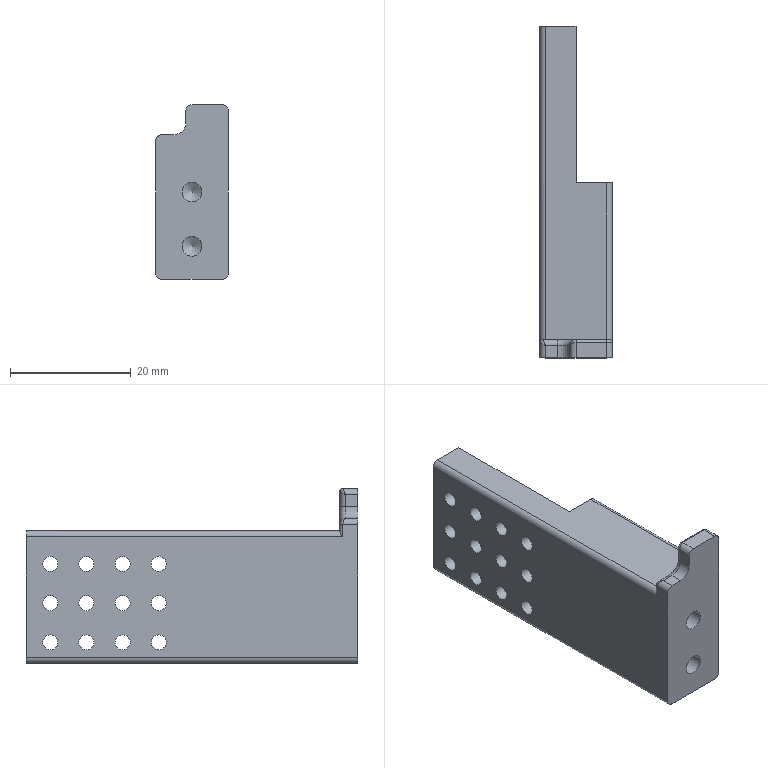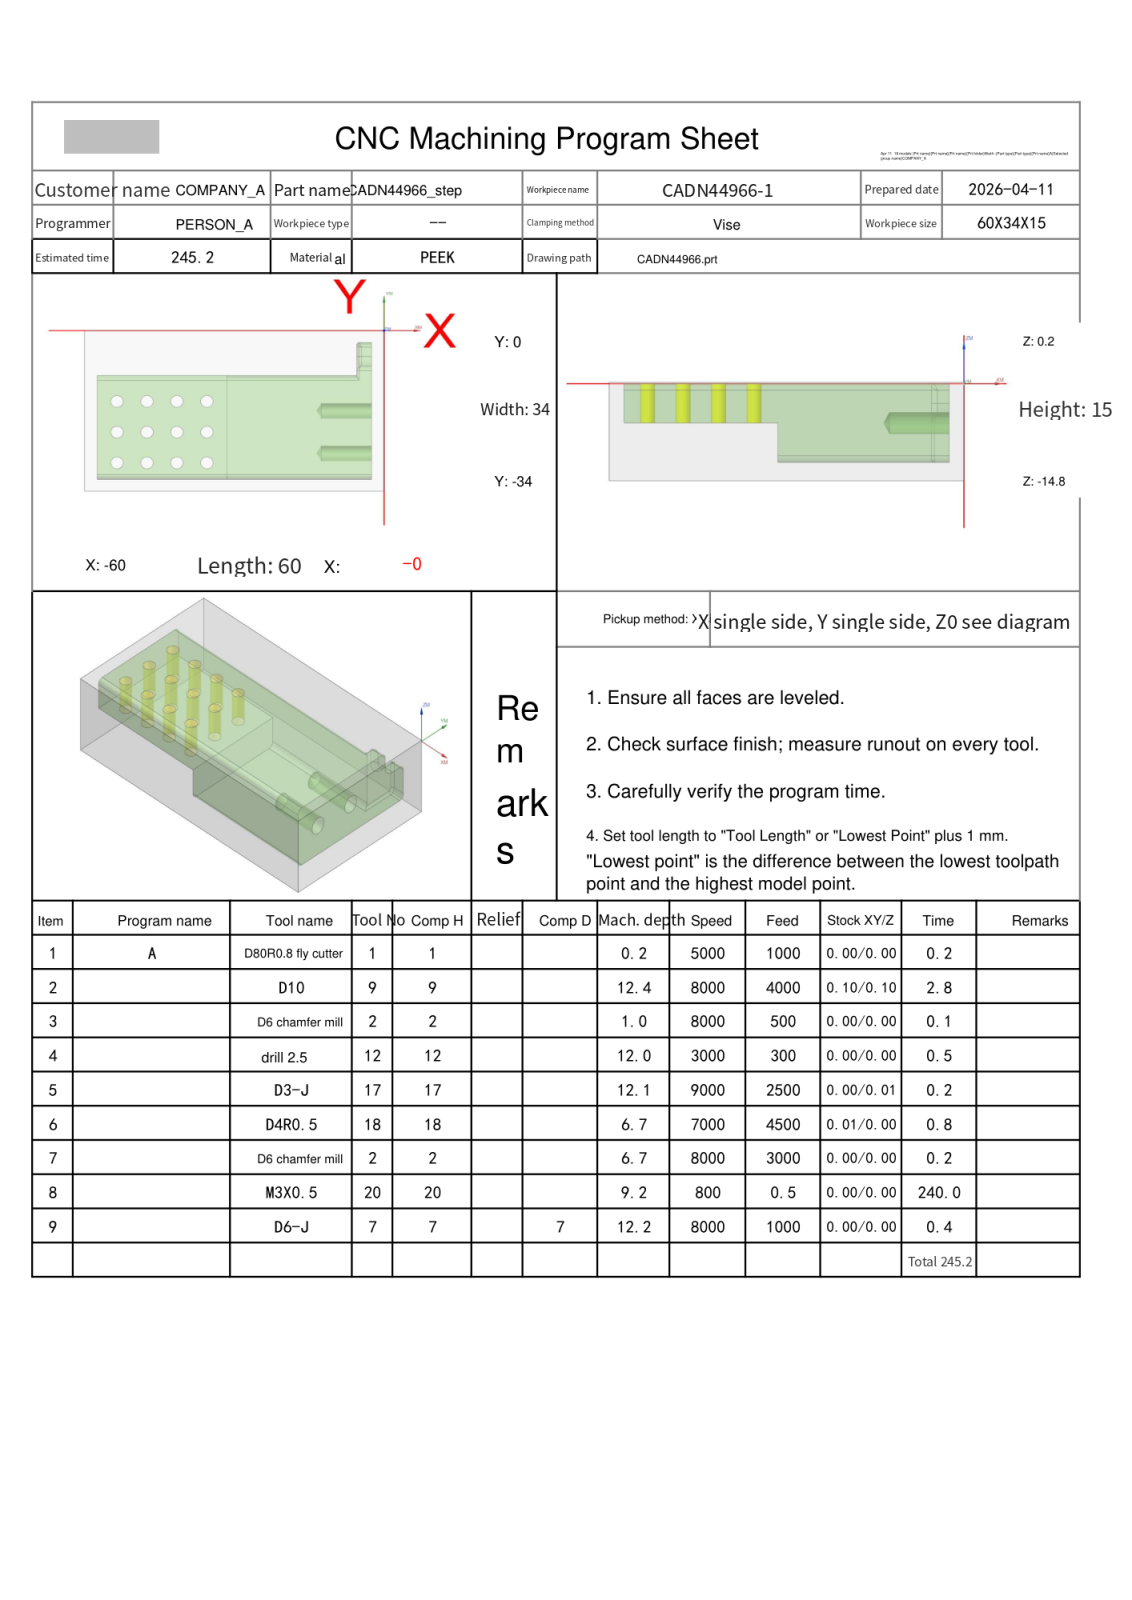NC program | NX | posted by the shop | part box 12 x 55 x 29 mm
Lines 1 to 2144 of 3281, first 1696 of 2142 lines:
%
O0001
(Machine time: 462.89 MIN)
(===Total Tool:8===)
(T1=D80R0.8 fly cutter D=80.  R=0.8  D-  H01 Z=0.    )
(T9=D10     D=10.  R=0.   D-  H09 Z=-12.2 )
(T2=D6 chamfer mill   D=6.   R=0.   D-  H02 Z=-6.5  )
(T12=drill 2.5  D=2.5  DR_a=118 D-  H12 Z=-11.75)
(T17=D3-J   D=3.   R=0.   D-  H17 Z=-11.95)
(T18=D4R0.5 D=4.   R=0.5  D-  H18 Z=-6.5  )
(T20=M3X0.5 D=2.5  DR_a=180 D-  H20 Z=-9.   )
(T7=D6-J    D=6.   R=0.   D7  H07 Z=-12.  )
G80 G90 G17 G49 G40
G91 G28 Z0
M01
N1 T01 M06
(D80R0.8 fly cutter  D=80. R=0.8 H=01 ce=0.00 di=0.00)
G00 G90 G54 X42.5 Y-17. M03 S5000
G43 H01 Z20.
M08
Z2.
G01 Z0.0 F1000.
X37.5
X-97.5
X-102.5
Z2.
G00 Z20.
G91 G28 Z0.0
M05
M09
G91 G28 Z0.0
M01
N2 T09 M06
(D10  D=10. R=0. H=09 ce=0.10 di=0.10)
G00 G90 G54 X-23.004 Y-46. M03 S8000
G43 H09 Z10.2
M08
Z.712
G01 Z-.488 F4000.
Y-44.874
G03 X-30.004 Y-37.874 I-7. J0.0
G01 X-57.509
G02 X-64. Y-31.341 I.041 J6.532
G01 Y-31.304
Y-9.696
Y-9.659
G02 X-60.5 Y-3.873 I6.533 J0.0
G01 Y0.0
G02 X-60. Y.5 I.5 J0.0
G01 X0.0
G02 X.5 Y0.0 I0.0 J-.5
G01 Y-1.869
G02 X4. Y-7.639 I-3.023 J-5.78
G01 Y-31.36
Y-31.367
G02 X-2.5 Y-37.874 I-6.506 J0.0
G01 X-35.004
G02 X-35.462 Y-37.511 I0.0 J.47
G01 X-35.524 Y-37.245
G03 X-36.497 Y-36.474 I-.974 J-.228
G01 X-57.5
G02 X-62.6 Y-31.341 I.033 J5.132
G01 Y-31.309
Y-9.692
Y-9.659
G02 X-57.5 Y-4.526 I5.133 J0.0
G01 X-9.108
G02 X-4.732 Y-2.526 I4.449 J-3.947
G01 X-2.5
G02 X2.6 Y-7.639 I-.023 J-5.123
G01 Y-31.361
Y-31.367
G02 X-2.5 Y-36.474 I-5.106 J0.0
G01 X-35.004
X-35.504
G03 X-42.504 Y-43.474 I0.0 J-7.
G01 Y-46.
Z.712
G00 Z3.
G01 X-23. F6000.
G00 Z.224
G01 Z-.976 F4000.
Y-45.
G03 X-30. Y-38. I-7. J0.0
G01 X-57.5
G02 X-64. Y-31.5 I0.0 J6.5
G01 Y-9.5
G02 X-60.5 Y-3.734 I6.5 J0.0
G01 Y0.0
G02 X-60. Y.5 I.5 J0.0
G01 X0.0
G02 X.5 Y0.0 I0.0 J-.5
G01 Y-1.735
G02 X4. Y-7.501 I-3.002 J-5.768
G01 Y-31.499
G02 X-2.5 Y-38. I-6.5 J0.0
G01 X-35.
G02 X-35.457 Y-37.637 I0.0 J.47
G01 X-35.519 Y-37.371
G03 X-36.493 Y-36.6 I-.974 J-.228
G01 X-57.5
G02 X-62.6 Y-31.5 I0.0 J5.1
G01 Y-9.5
G02 X-57.5 Y-4.4 I5.1 J0.0
G01 X-9.017
G02 X-4.793 Y-2.407 I4.517 J-4.1
G01 X-4.511 Y-2.4
X-2.504
X-2.502
G02 X2.6 Y-7.501 I0.0 J-5.102
G01 Y-31.499
G02 X-2.5 Y-36.6 I-5.1 J0.0
G01 X-35.
X-35.5
G03 X-42.5 Y-43.6 I0.0 J-7.
G01 Y-46.
Z.224
G00 Z2.512
G01 X-23. F6000.
G00 Z-.264
G01 Z-1.464 F4000.
Y-45.
G03 X-30. Y-38. I-7. J0.0
G01 X-57.5
G02 X-64. Y-31.5 I0.0 J6.5
G01 Y-9.5
G02 X-60.5 Y-3.734 I6.5 J0.0
G01 Y0.0
G02 X-60. Y.5 I.5 J0.0
G01 X0.0
G02 X.5 Y0.0 I0.0 J-.5
G01 Y-1.734
G02 X3.831 Y-6.028 I-3. J-5.766
X4. Y-7.5 I-6.331 J-1.472
G01 Y-31.5
G02 X-2.5 Y-38. I-6.5 J0.0
G01 X-35.
G02 X-35.457 Y-37.637 I0.0 J.47
G01 X-35.519 Y-37.372
G03 X-36.493 Y-36.6 I-.974 J-.228
G01 X-57.5
G02 X-62.6 Y-31.5 I0.0 J5.1
G01 Y-9.5
G02 X-57.5 Y-4.4 I5.1 J0.0
G01 X-9.017
G02 X-4.5 Y-2.4 I4.517 J-4.1
G01 X-2.5
G02 X-1.191 Y-2.571 I0.0 J-5.1
X2.467 Y-6.345 I-1.309 J-4.929
X2.6 Y-7.5 I-4.967 J-1.155
G01 Y-31.5
G02 X-2.5 Y-36.6 I-5.1 J0.0
G01 X-35.
X-35.5
G03 X-42.5 Y-43.6 I0.0 J-7.
G01 Y-46.
Z-.264
G00 Z2.024
G01 X-23. F6000.
G00 Z-.752
G01 Z-1.952 F4000.
Y-45.
G03 X-30. Y-38. I-7. J0.0
G01 X-57.5
G02 X-64. Y-31.5 I0.0 J6.5
G01 Y-9.5
G02 X-60.5 Y-3.734 I6.5 J0.0
G01 Y0.0
G02 X-60. Y.5 I.5 J0.0
G01 X0.0
G02 X.5 Y0.0 I0.0 J-.5
G01 Y-1.734
G02 X3.831 Y-6.028 I-3. J-5.766
X4. Y-7.5 I-6.331 J-1.472
G01 Y-31.5
G02 X-2.5 Y-38. I-6.5 J0.0
G01 X-35.
G02 X-35.457 Y-37.637 I0.0 J.47
G01 X-35.519 Y-37.372
G03 X-36.493 Y-36.6 I-.974 J-.228
G01 X-57.5
G02 X-62.6 Y-31.5 I0.0 J5.1
G01 Y-9.5
G02 X-57.5 Y-4.4 I5.1 J0.0
G01 X-9.017
G02 X-4.5 Y-2.4 I4.517 J-4.1
G01 X-2.5
G02 X-1.191 Y-2.571 I0.0 J-5.1
X2.467 Y-6.345 I-1.309 J-4.929
X2.6 Y-7.5 I-4.967 J-1.155
G01 Y-31.5
G02 X-2.5 Y-36.6 I-5.1 J0.0
G01 X-35.
X-35.5
G03 X-42.5 Y-43.6 I0.0 J-7.
G01 Y-46.
Z-.752
G00 Z1.536
G01 X-23. F6000.
G00 Z-1.24
G01 Z-2.44 F4000.
Y-45.
G03 X-30. Y-38. I-7. J0.0
G01 X-57.5
G02 X-64. Y-31.5 I0.0 J6.5
G01 Y-9.5
G02 X-60.5 Y-3.734 I6.5 J0.0
G01 Y0.0
G02 X-60. Y.5 I.5 J0.0
G01 X0.0
G02 X.5 Y0.0 I0.0 J-.5
G01 Y-1.734
G02 X3.831 Y-6.028 I-3. J-5.766
X4. Y-7.5 I-6.331 J-1.472
G01 Y-31.5
G02 X-2.5 Y-38. I-6.5 J0.0
G01 X-35.
G02 X-35.457 Y-37.637 I0.0 J.47
G01 X-35.519 Y-37.372
G03 X-36.493 Y-36.6 I-.974 J-.228
G01 X-57.5
G02 X-62.6 Y-31.5 I0.0 J5.1
G01 Y-9.5
G02 X-57.5 Y-4.4 I5.1 J0.0
G01 X-9.017
G02 X-4.5 Y-2.4 I4.517 J-4.1
G01 X-2.5
G02 X-1.191 Y-2.571 I0.0 J-5.1
X2.467 Y-6.345 I-1.309 J-4.929
X2.6 Y-7.5 I-4.967 J-1.155
G01 Y-31.5
G02 X-2.5 Y-36.6 I-5.1 J0.0
G01 X-35.
X-35.5
G03 X-42.5 Y-43.6 I0.0 J-7.
G01 Y-46.
Z-1.24
G00 Z1.048
G01 X-23. F6000.
G00 Z-1.728
G01 Z-2.928 F4000.
Y-45.
G03 X-30. Y-38. I-7. J0.0
G01 X-57.5
G02 X-64. Y-31.5 I0.0 J6.5
G01 Y-9.5
G02 X-60.5 Y-3.734 I6.5 J0.0
G01 Y0.0
G02 X-60. Y.5 I.5 J0.0
G01 X0.0
G02 X.5 Y0.0 I0.0 J-.5
G01 Y-1.734
G02 X3.831 Y-6.028 I-3. J-5.766
X4. Y-7.5 I-6.331 J-1.472
G01 Y-31.5
G02 X-2.5 Y-38. I-6.5 J0.0
G01 X-35.
G02 X-35.457 Y-37.637 I0.0 J.47
G01 X-35.519 Y-37.372
G03 X-36.493 Y-36.6 I-.974 J-.228
G01 X-57.5
G02 X-62.6 Y-31.5 I0.0 J5.1
G01 Y-9.5
G02 X-57.5 Y-4.4 I5.1 J0.0
G01 X-9.017
G02 X-4.5 Y-2.4 I4.517 J-4.1
G01 X-2.5
G02 X-1.191 Y-2.571 I0.0 J-5.1
X2.467 Y-6.345 I-1.309 J-4.929
X2.6 Y-7.5 I-4.967 J-1.155
G01 Y-31.5
G02 X-2.5 Y-36.6 I-5.1 J0.0
G01 X-35.
X-35.5
G03 X-42.5 Y-43.6 I0.0 J-7.
G01 Y-46.
Z-1.728
G00 Z.56
G01 X-23. F6000.
G00 Z-2.216
G01 Z-3.416 F4000.
Y-45.
G03 X-30. Y-38. I-7. J0.0
G01 X-57.5
G02 X-64. Y-31.5 I0.0 J6.5
G01 Y-9.5
G02 X-60.5 Y-3.734 I6.5 J0.0
G01 Y0.0
G02 X-60. Y.5 I.5 J0.0
G01 X0.0
G02 X.5 Y0.0 I0.0 J-.5
G01 Y-1.663
G02 X3.108 Y-4.152 I-2.927 J-5.678
X4. Y-7.413 I-5.511 J-3.261
G01 Y-7.459
Y-31.5
G02 X-2.5 Y-38. I-6.5 J0.0
G01 X-35.
G02 X-35.457 Y-37.637 I0.0 J.47
G01 X-35.519 Y-37.372
G03 X-36.493 Y-36.6 I-.974 J-.228
G01 X-57.5
G02 X-62.6 Y-31.5 I0.0 J5.1
G01 Y-9.5
G02 X-57.5 Y-4.4 I5.1 J0.0
G01 X-9.053
G02 X-4.523 Y-2.354 I4.53 J-3.991
G01 X-4.5
X-2.5
X-2.427 Y-2.353
G02 X1.899 Y-4.858 I0.0 J-4.988
X2.6 Y-7.413 I-4.302 J-2.555
G01 Y-7.454
Y-31.5
G02 X-2.5 Y-36.6 I-5.1 J0.0
G01 X-35.
X-35.5
G03 X-42.5 Y-43.6 I0.0 J-7.
G01 Y-46.
Z-2.216
G00 Z.072
G01 X-23. F6000.
G00 Z-2.704
G01 Z-3.904 F4000.
Y-45.
G03 X-30. Y-38. I-7. J0.0
G01 X-57.5
G02 X-64. Y-31.5 I0.0 J6.5
G01 Y-9.5
G02 X-60.5 Y-3.734 I6.5 J0.0
G01 Y0.0
G02 X-60. Y.5 I.5 J0.0
G01 X0.0
G02 X.5 Y0.0 I0.0 J-.5
G01 Y-1.486
G02 X4.003 Y-7.256 I-3. J-5.77
G01 X4. Y-7.454
Y-31.5
G02 X-2.5 Y-38. I-6.5 J0.0
G01 X-35.
G02 X-35.457 Y-37.637 I0.0 J.47
G01 X-35.519 Y-37.372
G03 X-36.493 Y-36.6 I-.974 J-.228
G01 X-57.5
G02 X-62.6 Y-31.5 I0.0 J5.1
G01 Y-9.5
G02 X-57.5 Y-4.4 I5.1 J0.0
G01 X-9.194
G02 X-4.516 Y-2.171 I4.678 J-3.795
G01 X-4.5
X-2.5
X-2.46 Y-2.148
X-1.864 Y-2.192
G02 X-.146 Y-2.728 I-.636 J-5.06
X2.604 Y-7.257 I-2.354 J-4.529
G01 X2.6 Y-7.454
Y-31.5
G02 X-2.5 Y-36.6 I-5.1 J0.0
G01 X-35.
X-35.5
G03 X-42.5 Y-43.6 I0.0 J-7.
G01 Y-46.
Z-2.704
G00 Z-.416
G01 X-23. F6000.
G00 Z-3.192
G01 Z-4.392 F4000.
Y-45.
G03 X-30. Y-38. I-7. J0.0
G01 X-57.5
G02 X-64. Y-31.5 I0.0 J6.5
G01 Y-9.5
G02 X-60.5 Y-3.734 I6.5 J0.0
G01 Y0.0
G02 X-60. Y.5 I.5 J0.0
G01 X0.0
G02 X.5 Y0.0 I0.0 J-.5
G01 Y-1.116
G02 X4. Y-6.867 I-2.974 J-5.751
G01 Y-6.941
Y-31.5
G02 X-2.5 Y-38. I-6.5 J0.0
G01 X-35.
G02 X-35.457 Y-37.637 I0.0 J.47
G01 X-35.519 Y-37.372
G03 X-36.493 Y-36.6 I-.974 J-.228
G01 X-57.5
G02 X-62.6 Y-31.5 I0.0 J5.1
G01 Y-9.5
G02 X-57.5 Y-4.4 I5.1 J0.0
G01 X-9.402
G02 X-4.543 Y-1.793 I4.859 J-3.225
G01 X-4.5
X-2.5
X-2.474
G02 X2.6 Y-6.867 I0.0 J-5.074
G01 Y-6.932
Y-31.5
G02 X-2.5 Y-36.6 I-5.1 J0.0
G01 X-35.
X-35.5
G03 X-42.5 Y-43.6 I0.0 J-7.
G01 Y-46.
Z-3.192
G00 Z-.904
G01 X-23. F6000.
G00 Z-3.68
G01 Z-4.88 F4000.
Y-45.
G03 X-30. Y-38. I-7. J0.0
G01 X-57.5
G02 X-64. Y-31.5 I0.0 J6.5
G01 Y-9.5
G02 X-60.5 Y-3.734 I6.5 J0.0
G01 Y0.0
G02 X-60. Y.5 I.5 J0.0
G01 X-5.654
G02 X-4.5 Y.625 I1.361 J-7.172
G01 X-2.462
G02 X-1.349 Y.5 I-.18 J-6.642
G01 X0.0
G02 X.5 Y0.0 I0.0 J-.5
G01 Y-.163
G02 X4.002 Y-6.017 I-3.142 J-5.854
G01 X4. Y-6.177
Y-31.5
G02 X-2.5 Y-38. I-6.5 J0.0
G01 X-35.
G02 X-35.457 Y-37.637 I0.0 J.47
G01 X-35.519 Y-37.372
G03 X-36.493 Y-36.6 I-.974 J-.228
G01 X-57.5
G02 X-62.6 Y-31.5 I0.0 J5.1
G01 Y-9.5
G02 X-57.5 Y-4.4 I5.1 J0.0
G01 X-9.734
G02 X-4.5 Y-.775 I5.446 J-2.272
G01 X-2.5
G02 X2.602 Y-6.017 I-.142 J-5.242
G01 X2.6 Y-6.159
Y-31.5
G02 X-2.5 Y-36.6 I-5.1 J0.0
G01 X-35.
X-35.5
G03 X-42.5 Y-43.6 I0.0 J-7.
G01 Y-46.
Z-3.68
G00 Z-1.392
G01 X-23. F6000.
G00 Z-4.168
G01 Z-5.368 F4000.
Y-45.
G03 X-30. Y-38. I-7. J0.0
G01 X-57.5
G02 X-64. Y-31.5 I0.0 J6.5
G01 Y-9.5
G02 X-60.5 Y-3.734 I6.5 J0.0
G01 Y0.0
G02 X-60. Y.5 I.5 J0.0
G01 X-10.791
G02 X-4.909 Y3.8 I5.882 J-3.591
G01 X-2.497
G02 X4. Y-2.712 I-.016 J-6.513
G01 Y-2.727
Y-5.857
X4.002 Y-6.017
X4. Y-6.177
Y-31.5
G02 X-2.5 Y-38. I-6.5 J0.0
G01 X-35.
G02 X-35.457 Y-37.637 I0.0 J.47
G01 X-35.519 Y-37.372
G03 X-36.493 Y-36.6 I-.974 J-.228
G01 X-57.5
G02 X-62.6 Y-31.5 I0.0 J5.1
G01 Y-9.5
G02 X-57.5 Y-4.4 I5.1 J0.0
G01 X-10.4
Y-3.091
G02 X-4.909 Y2.4 I5.492 J0.0
G01 X-2.5
G02 X2.6 Y-2.712 I-.013 J-5.113
G01 Y-2.725
Y-5.875
X2.602 Y-6.017
X2.6 Y-6.159
Y-31.5
G02 X-2.5 Y-36.6 I-5.1 J0.0
G01 X-35.
X-35.5
G03 X-42.5 Y-43.6 I0.0 J-7.
G01 Y-46.
Z-4.168
G00 Z-1.88
G01 X-23. F6000.
G00 Z-4.656
G01 Z-5.856 F4000.
Y-45.
G03 X-30. Y-38. I-7. J0.0
G01 X-57.5
G02 X-64. Y-31.5 I0.0 J6.5
G01 Y-9.5
G02 X-60.5 Y-3.734 I6.5 J0.0
G01 Y0.0
G02 X-60. Y.5 I.5 J0.0
G01 X-11.029
G02 X-4.996 Y3.991 I6.083 J-3.554
G01 X-2.5
G02 X4. Y-2.51 I0.0 J-6.5
G01 Y-5.857
X4.002 Y-6.017
X4. Y-6.177
Y-31.5
G02 X-2.5 Y-38. I-6.5 J0.0
G01 X-35.
G02 X-35.457 Y-37.637 I0.0 J.47
G01 X-35.519 Y-37.372
G03 X-36.493 Y-36.6 I-.974 J-.228
G01 X-57.5
G02 X-62.6 Y-31.5 I0.0 J5.1
G01 Y-9.5
G02 X-57.5 Y-4.4 I5.1 J0.0
G01 X-10.591
Y-3.004
G02 X-4.996 Y2.591 I5.645 J-.05
G01 X-2.5
G02 X2.6 Y-2.51 I0.0 J-5.1
G01 Y-5.875
X2.602 Y-6.017
X2.6 Y-6.159
Y-31.5
G02 X-2.5 Y-36.6 I-5.1 J0.0
G01 X-35.
X-35.5
G03 X-42.5 Y-43.6 I0.0 J-7.
G01 Y-46.
Z-4.656
G00 Z-2.368
G01 X-23. F6000.
G00 Z-5.144
G01 Z-6.344 F4000.
Y-45.
G03 X-30. Y-38. I-7. J0.0
G01 X-57.5
G02 X-64. Y-31.5 I0.0 J6.5
G01 Y-9.5
G02 X-60.5 Y-3.734 I6.5 J0.0
G01 Y0.0
G02 X-60. Y.5 I.5 J0.0
G01 X-11.062
G02 X-5. Y4. I6.062 J-3.5
G01 X-2.5
G02 X4. Y-2.5 I0.0 J-6.5
G01 Y-31.5
G02 X-2.5 Y-38. I-6.5 J0.0
G01 X-35.
G02 X-35.457 Y-37.637 I0.0 J.47
G01 X-35.519 Y-37.372
G03 X-36.493 Y-36.6 I-.974 J-.228
G01 X-57.5
G02 X-62.6 Y-31.5 I0.0 J5.1
G01 Y-9.5
G02 X-57.5 Y-4.4 I5.1 J0.0
G01 X-10.6
Y-3.
G02 X-5. Y2.6 I5.6 J0.0
G01 X-2.5
G02 X2.6 Y-2.5 I0.0 J-5.1
G01 Y-31.5
G02 X-2.5 Y-36.6 I-5.1 J0.0
G01 X-35.
X-35.5
G03 X-42.5 Y-43.6 I0.0 J-7.
G01 Y-46.
Z-5.144
G00 Z-2.856
G01 X-23. F6000.
G00 Z-5.632
G01 Z-6.832 F4000.
Y-45.
G03 X-30. Y-38. I-7. J0.0
G01 X-57.5
G02 X-64. Y-31.5 I0.0 J6.5
G01 Y-9.5
G02 X-60.5 Y-3.734 I6.5 J0.0
G01 Y0.0
G02 X-60. Y.5 I.5 J0.0
G01 X-11.062
G02 X-5. Y4. I6.062 J-3.5
G01 X-2.5
G02 X4. Y-2.5 I0.0 J-6.5
G01 Y-31.5
G02 X-2.5 Y-38. I-6.5 J0.0
G01 X-35.
G02 X-35.457 Y-37.637 I0.0 J.47
G01 X-35.519 Y-37.372
G03 X-36.493 Y-36.6 I-.974 J-.228
G01 X-57.5
G02 X-62.6 Y-31.5 I0.0 J5.1
G01 Y-9.5
G02 X-57.5 Y-4.4 I5.1 J0.0
G01 X-10.6
Y-3.
G02 X-5. Y2.6 I5.6 J0.0
G01 X-2.5
G02 X2.6 Y-2.5 I0.0 J-5.1
G01 Y-31.5
G02 X-2.5 Y-36.6 I-5.1 J0.0
G01 X-35.
X-35.5
G03 X-42.5 Y-43.6 I0.0 J-7.
G01 Y-46.
Z-5.632
G00 Z-3.344
G01 X-23. F6000.
G00 Z-6.12
G01 Z-7.32 F4000.
Y-45.
G03 X-30. Y-38. I-7. J0.0
G01 X-57.5
G02 X-64. Y-31.5 I0.0 J6.5
G01 Y-9.5
G02 X-60.5 Y-3.734 I6.5 J0.0
G01 Y0.0
G02 X-60. Y.5 I.5 J0.0
G01 X-11.062
G02 X-5. Y4. I6.062 J-3.5
G01 X-2.5
G02 X4. Y-2.5 I0.0 J-6.5
G01 Y-31.5
G02 X-2.5 Y-38. I-6.5 J0.0
G01 X-35.
G02 X-35.457 Y-37.637 I0.0 J.47
G01 X-35.519 Y-37.372
G03 X-36.493 Y-36.6 I-.974 J-.228
G01 X-57.5
G02 X-62.6 Y-31.5 I0.0 J5.1
G01 Y-9.5
G02 X-57.5 Y-4.4 I5.1 J0.0
G01 X-10.6
Y-3.
G02 X-5. Y2.6 I5.6 J0.0
G01 X-2.5
G02 X2.6 Y-2.5 I0.0 J-5.1
G01 Y-31.5
G02 X-2.5 Y-36.6 I-5.1 J0.0
G01 X-35.
X-35.5
G03 X-42.5 Y-43.6 I0.0 J-7.
G01 Y-46.
Z-6.12
G00 Z-3.832
G01 X-23. F6000.
G00 Z-6.608
G01 Z-7.808 F4000.
Y-45.
G03 X-30. Y-38. I-7. J0.0
G01 X-57.5
G02 X-64. Y-31.5 I0.0 J6.5
G01 Y-9.5
G02 X-60.5 Y-3.734 I6.5 J0.0
G01 Y0.0
G02 X-60. Y.5 I.5 J0.0
G01 X-11.062
G02 X-5. Y4. I6.062 J-3.5
G01 X-2.5
G02 X4. Y-2.5 I0.0 J-6.5
G01 Y-31.5
G02 X-2.5 Y-38. I-6.5 J0.0
G01 X-35.
G02 X-35.457 Y-37.637 I0.0 J.47
G01 X-35.519 Y-37.372
G03 X-36.493 Y-36.6 I-.974 J-.228
G01 X-57.5
G02 X-62.6 Y-31.5 I0.0 J5.1
G01 Y-9.5
G02 X-57.5 Y-4.4 I5.1 J0.0
G01 X-10.6
Y-3.
G02 X-5. Y2.6 I5.6 J0.0
G01 X-2.5
G02 X2.6 Y-2.5 I0.0 J-5.1
G01 Y-31.5
G02 X-2.5 Y-36.6 I-5.1 J0.0
G01 X-35.
X-35.5
G03 X-42.5 Y-43.6 I0.0 J-7.
G01 Y-46.
Z-6.608
G00 Z-4.32
G01 X-23. F6000.
G00 Z-7.096
G01 Z-8.296 F4000.
Y-45.
G03 X-30. Y-38. I-7. J0.0
G01 X-57.5
G02 X-64. Y-31.5 I0.0 J6.5
G01 Y-9.5
G02 X-60.5 Y-3.734 I6.5 J0.0
G01 Y0.0
G02 X-60. Y.5 I.5 J0.0
G01 X-11.062
G02 X-5. Y4. I6.062 J-3.5
G01 X-2.5
G02 X4. Y-2.5 I0.0 J-6.5
G01 Y-31.5
G02 X-2.5 Y-38. I-6.5 J0.0
G01 X-35.
G02 X-35.457 Y-37.637 I0.0 J.47
G01 X-35.519 Y-37.372
G03 X-36.493 Y-36.6 I-.974 J-.228
G01 X-57.5
G02 X-62.6 Y-31.5 I0.0 J5.1
G01 Y-9.5
G02 X-57.5 Y-4.4 I5.1 J0.0
G01 X-10.6
Y-3.
G02 X-5. Y2.6 I5.6 J0.0
G01 X-2.5
G02 X2.6 Y-2.5 I0.0 J-5.1
G01 Y-31.5
G02 X-2.5 Y-36.6 I-5.1 J0.0
G01 X-35.
X-35.5
G03 X-42.5 Y-43.6 I0.0 J-7.
G01 Y-46.
Z-7.096
G00 Z-4.808
G01 X-23. F6000.
G00 Z-7.584
G01 Z-8.784 F4000.
Y-45.
G03 X-30. Y-38. I-7. J0.0
G01 X-57.5
G02 X-64. Y-31.5 I0.0 J6.5
G01 Y-9.5
G02 X-60.5 Y-3.734 I6.5 J0.0
G01 Y0.0
G02 X-60. Y.5 I.5 J0.0
G01 X-11.062
G02 X-5. Y4. I6.062 J-3.5
G01 X-2.5
G02 X4. Y-2.5 I0.0 J-6.5
G01 Y-31.5
G02 X-2.5 Y-38. I-6.5 J0.0
G01 X-35.
G02 X-35.457 Y-37.637 I0.0 J.47
G01 X-35.519 Y-37.372
G03 X-36.493 Y-36.6 I-.974 J-.228
G01 X-57.5
G02 X-62.6 Y-31.5 I0.0 J5.1
G01 Y-9.5
G02 X-57.5 Y-4.4 I5.1 J0.0
G01 X-10.6
Y-3.
G02 X-5. Y2.6 I5.6 J0.0
G01 X-2.5
G02 X2.6 Y-2.5 I0.0 J-5.1
G01 Y-31.5
G02 X-2.5 Y-36.6 I-5.1 J0.0
G01 X-35.
X-35.5
G03 X-42.5 Y-43.6 I0.0 J-7.
G01 Y-46.
Z-7.584
G00 Z-5.296
G01 X-23. F6000.
G00 Z-8.072
G01 Z-9.272 F4000.
Y-45.
G03 X-30. Y-38. I-7. J0.0
G01 X-57.5
G02 X-64. Y-31.5 I0.0 J6.5
G01 Y-9.5
G02 X-60.5 Y-3.734 I6.5 J0.0
G01 Y0.0
G02 X-60. Y.5 I.5 J0.0
G01 X-11.062
G02 X-5. Y4. I6.062 J-3.5
G01 X-2.5
G02 X4. Y-2.5 I0.0 J-6.5
G01 Y-31.5
G02 X-2.5 Y-38. I-6.5 J0.0
G01 X-35.
G02 X-35.457 Y-37.637 I0.0 J.47
G01 X-35.519 Y-37.372
G03 X-36.493 Y-36.6 I-.974 J-.228
G01 X-57.5
G02 X-62.6 Y-31.5 I0.0 J5.1
G01 Y-9.5
G02 X-57.5 Y-4.4 I5.1 J0.0
G01 X-10.6
Y-3.
G02 X-5. Y2.6 I5.6 J0.0
G01 X-2.5
G02 X2.6 Y-2.5 I0.0 J-5.1
G01 Y-31.5
G02 X-2.5 Y-36.6 I-5.1 J0.0
G01 X-35.
X-35.5
G03 X-42.5 Y-43.6 I0.0 J-7.
G01 Y-46.
Z-8.072
G00 Z-5.784
G01 X-23. F6000.
G00 Z-8.56
G01 Z-9.76 F4000.
Y-45.
G03 X-30. Y-38. I-7. J0.0
G01 X-57.5
G02 X-64. Y-31.5 I0.0 J6.5
G01 Y-9.5
G02 X-60.5 Y-3.734 I6.5 J0.0
G01 Y0.0
G02 X-60. Y.5 I.5 J0.0
G01 X-11.062
G02 X-5. Y4. I6.062 J-3.5
G01 X-2.5
G02 X4. Y-2.5 I0.0 J-6.5
G01 Y-31.5
G02 X-2.5 Y-38. I-6.5 J0.0
G01 X-35.
G02 X-35.457 Y-37.637 I0.0 J.47
G01 X-35.519 Y-37.372
G03 X-36.493 Y-36.6 I-.974 J-.228
G01 X-57.5
G02 X-62.6 Y-31.5 I0.0 J5.1
G01 Y-9.5
G02 X-57.5 Y-4.4 I5.1 J0.0
G01 X-10.6
Y-3.
G02 X-5. Y2.6 I5.6 J0.0
G01 X-2.5
G02 X2.6 Y-2.5 I0.0 J-5.1
G01 Y-31.5
G02 X-2.5 Y-36.6 I-5.1 J0.0
G01 X-35.
X-35.5
G03 X-42.5 Y-43.6 I0.0 J-7.
G01 Y-46.
Z-8.56
G00 Z-6.272
G01 X-23. F6000.
G00 Z-9.048
G01 Z-10.248 F4000.
Y-45.
G03 X-30. Y-38. I-7. J0.0
G01 X-57.5
G02 X-64. Y-31.5 I0.0 J6.5
G01 Y-9.5
G02 X-60.5 Y-3.734 I6.5 J0.0
G01 Y0.0
G02 X-60. Y.5 I.5 J0.0
G01 X-11.062
G02 X-5. Y4. I6.062 J-3.5
G01 X-2.5
G02 X4. Y-2.5 I0.0 J-6.5
G01 Y-31.5
G02 X-2.5 Y-38. I-6.5 J0.0
G01 X-35.
G02 X-35.457 Y-37.637 I0.0 J.47
G01 X-35.519 Y-37.372
G03 X-36.493 Y-36.6 I-.974 J-.228
G01 X-57.5
G02 X-62.6 Y-31.5 I0.0 J5.1
G01 Y-9.5
G02 X-57.5 Y-4.4 I5.1 J0.0
G01 X-10.6
Y-3.
G02 X-5. Y2.6 I5.6 J0.0
G01 X-2.5
G02 X2.6 Y-2.5 I0.0 J-5.1
G01 Y-31.5
G02 X-2.5 Y-36.6 I-5.1 J0.0
G01 X-35.
X-35.5
G03 X-42.5 Y-43.6 I0.0 J-7.
G01 Y-46.
Z-9.048
G00 Z-6.76
G01 X-23. F6000.
G00 Z-9.536
G01 Z-10.736 F4000.
Y-45.
G03 X-30. Y-38. I-7. J0.0
G01 X-57.5
G02 X-64. Y-31.5 I0.0 J6.5
G01 Y-9.5
G02 X-60.5 Y-3.734 I6.5 J0.0
G01 Y0.0
G02 X-60. Y.5 I.5 J0.0
G01 X-11.062
G02 X-5. Y4. I6.062 J-3.5
G01 X-2.5
G02 X4. Y-2.5 I0.0 J-6.5
G01 Y-31.5
G02 X-2.5 Y-38. I-6.5 J0.0
G01 X-35.
G02 X-35.457 Y-37.637 I0.0 J.47
G01 X-35.519 Y-37.372
G03 X-36.493 Y-36.6 I-.974 J-.228
G01 X-57.5
G02 X-62.6 Y-31.5 I0.0 J5.1
G01 Y-9.5
G02 X-57.5 Y-4.4 I5.1 J0.0
G01 X-10.6
Y-3.
G02 X-5. Y2.6 I5.6 J0.0
G01 X-2.5
G02 X2.6 Y-2.5 I0.0 J-5.1
G01 Y-31.5
G02 X-2.5 Y-36.6 I-5.1 J0.0
G01 X-35.
X-35.5
G03 X-42.5 Y-43.6 I0.0 J-7.
G01 Y-46.
Z-9.536
G00 Z-7.248
G01 X-23. F6000.
G00 Z-10.024
G01 Z-11.224 F4000.
Y-45.
G03 X-30. Y-38. I-7. J0.0
G01 X-57.5
G02 X-64. Y-31.5 I0.0 J6.5
G01 Y-9.5
G02 X-60.5 Y-3.734 I6.5 J0.0
G01 Y0.0
G02 X-60. Y.5 I.5 J0.0
G01 X-11.062
G02 X-5. Y4. I6.062 J-3.5
G01 X-4.943
X-2.5
G02 X4. Y-2.5 I0.0 J-6.5
G01 Y-31.5
G02 X-2.5 Y-38. I-6.5 J0.0
G01 X-35.
G02 X-35.457 Y-37.637 I0.0 J.47
G01 X-35.519 Y-37.372
G03 X-36.493 Y-36.6 I-.974 J-.228
G01 X-57.5
G02 X-62.6 Y-31.5 I0.0 J5.1
G01 Y-9.5
G02 X-57.5 Y-4.4 I5.1 J0.0
G01 X-10.6
Y-3.
G02 X-9.85 Y-.2 I5.6 J0.0
X-5. Y2.6 I4.85 J-2.8
G01 X-4.943
X-2.5
G02 X2.6 Y-2.5 I0.0 J-5.1
G01 Y-31.5
G02 X-2.5 Y-36.6 I-5.1 J0.0
G01 X-35.
X-35.5
G03 X-42.5 Y-43.6 I0.0 J-7.
G01 Y-46.
Z-10.024
G00 Z-7.736
G01 X-23. F6000.
G00 Z-10.512
G01 Z-11.712 F4000.
Y-45.
G03 X-30. Y-38. I-7. J0.0
G01 X-57.5
G02 X-64. Y-31.5 I0.0 J6.5
G01 Y-9.5
G02 X-60.5 Y-3.734 I6.5 J0.0
G01 Y0.0
G02 X-60. Y.5 I.5 J0.0
G01 X-11.062
G02 X-5. Y4. I6.062 J-3.5
G01 X-4.943
X-2.5
G02 X4. Y-2.5 I0.0 J-6.5
G01 Y-31.5
G02 X-2.5 Y-38. I-6.5 J0.0
G01 X-35.
G02 X-35.457 Y-37.637 I0.0 J.47
G01 X-35.519 Y-37.372
G03 X-36.493 Y-36.6 I-.974 J-.228
G01 X-57.5
G02 X-62.6 Y-31.5 I0.0 J5.1
G01 Y-9.5
G02 X-57.5 Y-4.4 I5.1 J0.0
G01 X-10.6
Y-3.
G02 X-9.85 Y-.2 I5.6 J0.0
X-5. Y2.6 I4.85 J-2.8
G01 X-4.943
X-2.5
G02 X2.6 Y-2.5 I0.0 J-5.1
G01 Y-31.5
G02 X-2.5 Y-36.6 I-5.1 J0.0
G01 X-35.
X-35.5
G03 X-42.5 Y-43.6 I0.0 J-7.
G01 Y-46.
Z-10.512
G00 Z-8.224
G01 X-23. F6000.
G00 Z-11.
G01 Z-12.2 F4000.
Y-45.
G03 X-30. Y-38. I-7. J0.0
G01 X-57.5
G02 X-64. Y-31.5 I0.0 J6.5
G01 Y-9.5
G02 X-60.5 Y-3.734 I6.5 J0.0
G01 Y0.0
G02 X-60. Y.5 I.5 J0.0
G01 X-11.062
G02 X-5. Y4. I6.062 J-3.5
G01 X-4.943
X-2.5
G02 X4. Y-2.5 I0.0 J-6.5
G01 Y-31.5
G02 X-2.5 Y-38. I-6.5 J0.0
G01 X-35.
G02 X-35.457 Y-37.637 I0.0 J.47
G01 X-35.519 Y-37.372
G03 X-36.493 Y-36.6 I-.974 J-.228
G01 X-57.5
G02 X-62.6 Y-31.5 I0.0 J5.1
G01 Y-9.5
G02 X-57.5 Y-4.4 I5.1 J0.0
G01 X-10.6
Y-3.
G02 X-9.85 Y-.2 I5.6 J0.0
X-5. Y2.6 I4.85 J-2.8
G01 X-4.943
X-2.5
G02 X2.6 Y-2.5 I0.0 J-5.1
G01 Y-31.5
G02 X-2.5 Y-36.6 I-5.1 J0.0
G01 X-35.
X-35.5
G03 X-42.5 Y-43.6 I0.0 J-7.
G01 Y-46.
Z-11.
G00 Z10.2
G91 G28 Z0.0
M05
M09
G91 G28 Z0.0
M01
N3 T02 M06
(D6 chamfer mill  D=6. R=0. H=02 ce=0.00 di=0.10)
G00 G90 G54 X-53.5 Y-15. M03 S8000
G43 H02 Z20.
M08
G98 G81 X-53.5 Y-15. Z-.8 R1. F500.
X-47.5
X-41.5
X-35.5
Y-21.5
X-41.5
X-47.5
X-53.5
Y-28.
X-47.5
X-41.5
X-35.5
G80
G00 Z20.
G91 G28 Z0.0
M05
M09
G91 G28 Z0.0
M01
N4 T12 M06
(drill 2.5 D=2.5 DR_a=118 H=12)
G00 G90 G54 X-53.5 Y-15. M03 S3000
G43 H12 Z20.
M08
G98 G83 X-53.5 Y-15. Z-11.751 R1. F300. Q2.
X-47.5
X-41.5
X-35.5
Y-21.5
X-41.5
X-47.5
X-53.5
Y-28.
X-47.5
X-41.5
X-35.5
G80
G00 Z20.
G91 G28 Z0.0
M05
M09
G91 G28 Z0.0
M01
N5 T17 M06
(D3-J  D=3. R=0. H=17 ce=0.00 di=0.01)
G00 G90 G54 X-9.532 Y-7.96 M03 S9000
G43 H17 Z20.
M08
Z.466
G01 X-9.531 Y-7.964 Z.393 F2000.
X-9.528 Y-7.976 Z.32
X-9.524 Y-7.994 Z.248
X-9.517 Y-8.017 Z.177
X-9.508 Y-8.044 Z.108
X-9.495 Y-8.074 Z.041
X-9.481 Y-8.105 Z-.022
X-9.463 Y-8.137 Z-.08
X-9.441 Y-8.169 Z-.133
X-9.416 Y-8.199 Z-.181
X-9.388 Y-8.226 Z-.221
X-9.355 Y-8.249 Z-.254
X-9.319 Y-8.267 Z-.278
X-9.278 Y-8.278 Z-.293
X-9.232 Y-8.282 Z-.299
X-6.947 F2500.
G02 X-6.246 Y-6.85 I2.2 J-.19
G01 X-6.23 Y-6.819 Z-.295
X-6.253 Y-6.793 Z-.286
X-6.311 Y-6.774 Z-.273
X-6.398 Y-6.761 Z-.256
X-6.51 Y-6.755 Z-.239
X-6.643 Y-6.756 Z-.221
X-6.791 Y-6.765 Z-.206
X-6.951 Y-6.783 Z-.194
X-7.118 Y-6.81 Z-.186
X-7.424 Y-6.88 Z-.187
X-7.731 Y-6.979 Z-.206
X-8.032 Y-7.103 Z-.241
X-8.321 Y-7.249 Z-.29
X-8.591 Y-7.417 Z-.349
X-8.717 Y-7.507 Z-.382
X-8.834 Y-7.599 Z-.415
X-8.941 Y-7.691 Z-.449
X-9.034 Y-7.778 Z-.482
X-9.113 Y-7.86 Z-.513
X-9.174 Y-7.933 Z-.541
X-9.215 Y-7.994 Z-.564
X-9.234 Y-8.041 Z-.582
X-9.23 Y-8.072 Z-.593
X-9.199 Y-8.082 Z-.598
X-6.965
G02 X-6.488 Y-6.984 I2.465 J-.418
X-6.214 Y-6.686 I1.828 J-1.402
G01 X-6.199 Y-6.657
X-6.216 Y-6.633 Z-.601
X-6.263 Y-6.613 Z-.604
X-6.336 Y-6.598 Z-.609
X-6.431 Y-6.588 Z-.615
X-6.544 Y-6.584 Z-.622
X-6.672 Y-6.587 Z-.63
X-6.811 Y-6.596 Z-.639
X-6.958 Y-6.613 Z-.649
X-7.109 Y-6.638 Z-.659
X-7.412 Y-6.712 Z-.682
X-7.711 Y-6.816 Z-.706
X-8.001 Y-6.949 Z-.733
X-8.278 Y-7.107 Z-.761
X-8.534 Y-7.287 Z-.79
X-8.654 Y-7.384 Z-.805
X-8.765 Y-7.484 Z-.82
X-8.866 Y-7.582 Z-.835
X-8.954 Y-7.677 Z-.849
X-9.028 Y-7.765 Z-.862
X-9.085 Y-7.844 Z-.873
X-9.123 Y-7.91 Z-.883
X-9.14 Y-7.961 Z-.89
X-9.133 Y-7.993 Z-.895
X-9.102 Y-8.005 Z-.896
X-6.95
G02 X-6.183 Y-6.651 I2.45 J-.495
G01 X-6.167 Y-6.623 Z-.897
X-6.185 Y-6.598 Z-.9
X-6.231 Y-6.578 Z-.905
X-6.303 Y-6.563 Z-.912
X-6.398 Y-6.553 Z-.92
X-6.51 Y-6.549 Z-.93
X-6.638 Y-6.552 Z-.94
X-6.777 Y-6.561 Z-.952
X-6.924 Y-6.578 Z-.964
X-7.076 Y-6.604 Z-.977
X-7.38 Y-6.68 Z-1.004
X-7.682 Y-6.787 Z-1.031
X-7.976 Y-6.923 Z-1.059
X-8.256 Y-7.084 Z-1.087
X-8.517 Y-7.269 Z-1.114
X-8.639 Y-7.368 Z-1.127
X-8.752 Y-7.469 Z-1.139
X-8.855 Y-7.57 Z-1.151
X-8.945 Y-7.666 Z-1.161
X-9.02 Y-7.756 Z-1.171
X-9.078 Y-7.836 Z-1.179
X-9.117 Y-7.903 Z-1.186
X-9.135 Y-7.955 Z-1.191
X-9.129 Y-7.988 Z-1.194
X-9.097 Y-8. Z-1.195
X-6.949
G02 X-6.181 Y-6.65 I2.449 J-.5
G01 X-6.165 Y-6.621 Z-1.196
X-6.182 Y-6.597 Z-1.199
X-6.227 Y-6.578 Z-1.204
X-6.298 Y-6.564 Z-1.211
X-6.391 Y-6.555 Z-1.219
X-6.503 Y-6.552 Z-1.228
X-6.629 Y-6.556 Z-1.239
X-6.767 Y-6.567 Z-1.25
X-6.913 Y-6.585 Z-1.262
X-7.063 Y-6.612 Z-1.275
X-7.368 Y-6.688 Z-1.302
X-7.67 Y-6.795 Z-1.33
X-7.966 Y-6.93 Z-1.358
X-8.248 Y-7.091 Z-1.385
X-8.511 Y-7.273 Z-1.412
X-8.633 Y-7.372 Z-1.425
X-8.747 Y-7.473 Z-1.438
X-8.851 Y-7.572 Z-1.449
X-8.942 Y-7.668 Z-1.46
X-9.018 Y-7.757 Z-1.47
X-9.077 Y-7.837 Z-1.478
X-9.116 Y-7.904 Z-1.484
X-9.134 Y-7.955 Z-1.489
X-9.129 Y-7.988 Z-1.493
X-9.097 Y-8. Z-1.494
X-6.949
G02 X-6.181 Y-6.65 I2.449 J-.5
G01 X-6.165 Y-6.621 Z-1.495
X-6.182 Y-6.597 Z-1.498
X-6.227 Y-6.578 Z-1.503
X-6.298 Y-6.564 Z-1.509
X-6.391 Y-6.555 Z-1.517
X-6.503 Y-6.552 Z-1.527
X-6.629 Y-6.556 Z-1.537
X-6.767 Y-6.567 Z-1.549
X-6.913 Y-6.585 Z-1.561
X-7.063 Y-6.612 Z-1.574
X-7.368 Y-6.688 Z-1.6
X-7.67 Y-6.795 Z-1.628
X-7.966 Y-6.93 Z-1.656
X-8.248 Y-7.091 Z-1.684
X-8.511 Y-7.273 Z-1.711
X-8.633 Y-7.372 Z-1.724
X-8.747 Y-7.473 Z-1.736
X-8.851 Y-7.572 Z-1.748
X-8.942 Y-7.668 Z-1.759
X-9.018 Y-7.757 Z-1.768
X-9.077 Y-7.837 Z-1.776
X-9.116 Y-7.904 Z-1.783
X-9.134 Y-7.955 Z-1.788
X-9.129 Y-7.988 Z-1.791
X-9.097 Y-8. Z-1.793
X-6.949
G02 X-6.181 Y-6.65 I2.449 J-.5
G01 X-6.165 Y-6.621 Z-1.794
X-6.182 Y-6.597 Z-1.797
X-6.227 Y-6.578 Z-1.801
X-6.298 Y-6.564 Z-1.808
X-6.391 Y-6.555 Z-1.816
X-6.503 Y-6.552 Z-1.825
X-6.629 Y-6.556 Z-1.836
X-6.767 Y-6.567 Z-1.847
X-6.913 Y-6.585 Z-1.859
X-7.063 Y-6.612 Z-1.872
X-7.368 Y-6.688 Z-1.899
X-7.67 Y-6.795 Z-1.926
X-7.966 Y-6.93 Z-1.955
X-8.248 Y-7.091 Z-1.982
X-8.511 Y-7.273 Z-2.01
X-8.633 Y-7.372 Z-2.023
X-8.747 Y-7.473 Z-2.035
X-8.851 Y-7.572 Z-2.047
X-8.942 Y-7.668 Z-2.057
X-9.018 Y-7.757 Z-2.067
X-9.077 Y-7.837 Z-2.075
X-9.116 Y-7.904 Z-2.082
X-9.134 Y-7.955 Z-2.087
X-9.129 Y-7.988 Z-2.09
X-9.097 Y-8. Z-2.091
X-6.949
G02 X-6.181 Y-6.65 I2.449 J-.5
G01 X-6.165 Y-6.621 Z-2.092
X-6.182 Y-6.597 Z-2.095
X-6.227 Y-6.578 Z-2.1
X-6.298 Y-6.564 Z-2.107
X-6.391 Y-6.555 Z-2.115
X-6.503 Y-6.552 Z-2.124
X-6.629 Y-6.556 Z-2.134
X-6.767 Y-6.567 Z-2.146
X-6.913 Y-6.585 Z-2.158
X-7.064 Y-6.612 Z-2.17
X-7.368 Y-6.688 Z-2.197
X-7.67 Y-6.795 Z-2.225
X-7.966 Y-6.93 Z-2.253
X-8.248 Y-7.091 Z-2.281
X-8.511 Y-7.273 Z-2.308
X-8.633 Y-7.372 Z-2.321
X-8.747 Y-7.473 Z-2.334
X-8.851 Y-7.572 Z-2.345
X-8.942 Y-7.668 Z-2.356
X-9.018 Y-7.757 Z-2.366
X-9.077 Y-7.837 Z-2.374
X-9.116 Y-7.904 Z-2.381
X-9.134 Y-7.955 Z-2.386
X-9.129 Y-7.988 Z-2.389
X-9.097 Y-8. Z-2.39
X-6.949
G02 X-6.181 Y-6.65 I2.449 J-.5
G01 X-6.165 Y-6.621 Z-2.391
X-6.182 Y-6.597 Z-2.394
X-6.227 Y-6.578 Z-2.399
X-6.298 Y-6.564 Z-2.405
X-6.391 Y-6.555 Z-2.413
X-6.503 Y-6.552 Z-2.422
X-6.629 Y-6.556 Z-2.433
X-6.767 Y-6.567 Z-2.444
X-6.913 Y-6.585 Z-2.456
X-7.064 Y-6.612 Z-2.469
X-7.368 Y-6.688 Z-2.495
X-7.671 Y-6.795 Z-2.523
X-7.966 Y-6.93 Z-2.551
X-8.248 Y-7.091 Z-2.579
X-8.511 Y-7.273 Z-2.607
X-8.633 Y-7.372 Z-2.62
X-8.748 Y-7.473 Z-2.632
X-8.851 Y-7.572 Z-2.644
X-8.942 Y-7.668 Z-2.655
X-9.018 Y-7.757 Z-2.664
X-9.077 Y-7.837 Z-2.673
X-9.116 Y-7.904 Z-2.679
X-9.134 Y-7.955 Z-2.684
X-9.129 Y-7.988 Z-2.688
X-9.097 Y-8. Z-2.689
X-6.949
G02 X-6.181 Y-6.65 I2.449 J-.5
G01 X-6.165 Y-6.621 Z-2.69
X-6.182 Y-6.597 Z-2.693
X-6.227 Y-6.578 Z-2.698
X-6.298 Y-6.564 Z-2.704
X-6.391 Y-6.555 Z-2.712
X-6.503 Y-6.552 Z-2.721
X-6.629 Y-6.556 Z-2.731
X-6.767 Y-6.567 Z-2.743
X-6.913 Y-6.585 Z-2.755
X-7.064 Y-6.612 Z-2.767
X-7.368 Y-6.688 Z-2.794
X-7.671 Y-6.795 Z-2.822
X-7.966 Y-6.93 Z-2.85
X-8.248 Y-7.091 Z-2.878
X-8.511 Y-7.273 Z-2.905
X-8.633 Y-7.372 Z-2.918
X-8.748 Y-7.473 Z-2.931
X-8.851 Y-7.572 Z-2.943
X-8.942 Y-7.668 Z-2.953
X-9.018 Y-7.757 Z-2.963
X-9.077 Y-7.837 Z-2.971
X-9.116 Y-7.904 Z-2.978
X-9.134 Y-7.955 Z-2.983
X-9.129 Y-7.988 Z-2.986
X-9.097 Y-8. Z-2.988
X-6.949
G02 X-6.181 Y-6.65 I2.449 J-.5
G01 X-6.165 Y-6.621 Z-2.989
X-6.182 Y-6.597 Z-2.992
X-6.228 Y-6.578 Z-2.996
X-6.299 Y-6.564 Z-3.003
X-6.393 Y-6.555 Z-3.01
X-6.505 Y-6.552 Z-3.02
X-6.632 Y-6.556 Z-3.03
X-6.771 Y-6.567 Z-3.041
X-6.918 Y-6.585 Z-3.053
X-7.069 Y-6.611 Z-3.066
X-7.375 Y-6.688 Z-3.092
X-7.679 Y-6.795 Z-3.12
X-7.976 Y-6.93 Z-3.148
X-8.26 Y-7.091 Z-3.176
X-8.525 Y-7.273 Z-3.204
X-8.648 Y-7.372 Z-3.217
X-8.763 Y-7.473 Z-3.229
X-8.867 Y-7.572 Z-3.241
X-8.959 Y-7.668 Z-3.252
X-9.036 Y-7.757 Z-3.262
X-9.095 Y-7.837 Z-3.27
X-9.135 Y-7.904 Z-3.277
X-9.153 Y-7.955 Z-3.282
X-9.148 Y-7.988 Z-3.285
X-9.117 Y-8. Z-3.286
X-6.954
X-6.92 Y-7.865
X-6.915 Y-7.853
X-6.873 Y-7.714
G02 X-6.403 Y-6.862 I2.075 J-.59
X-6.191 Y-6.64 I1.907 J-1.607
G01 X-6.175 Y-6.612 Z-3.287
X-6.193 Y-6.588 Z-3.289
X-6.24 Y-6.568 Z-3.292
X-6.312 Y-6.554 Z-3.297
X-6.407 Y-6.546 Z-3.303
X-6.521 Y-6.543 Z-3.31
X-6.649 Y-6.547 Z-3.318
X-6.79 Y-6.559 Z-3.328
X-6.938 Y-6.577 Z-3.338
X-7.091 Y-6.604 Z-3.349
X-7.4 Y-6.681 Z-3.375
X-7.708 Y-6.79 Z-3.403
X-8.008 Y-6.926 Z-3.433
X-8.295 Y-7.087 Z-3.464
X-8.562 Y-7.271 Z-3.494
X-8.687 Y-7.37 Z-3.509
X-8.803 Y-7.471 Z-3.522
X-8.908 Y-7.571 Z-3.535
X-9.001 Y-7.667 Z-3.547
X-9.079 Y-7.757 Z-3.558
X-9.139 Y-7.836 Z-3.567
X-9.179 Y-7.904 Z-3.575
X-9.198 Y-7.955 Z-3.58
X-9.193 Y-7.988 Z-3.584
X-9.162 Y-8. Z-3.585
X-6.964
G02 X-6.219 Y-6.606 I2.505 J-.442
G01 X-6.204 Y-6.576
X-6.223 Y-6.552 Z-3.584
X-6.272 Y-6.532
X-6.348 Y-6.518
X-6.446 Y-6.51 Z-3.585
X-6.563 Y-6.508 Z-3.586
X-6.695 Y-6.513 Z-3.589
X-6.839 Y-6.525 Z-3.594
X-6.991 Y-6.544 Z-3.6
X-7.147 Y-6.572 Z-3.608
X-7.463 Y-6.652 Z-3.631
X-7.776 Y-6.764 Z-3.661
X-8.08 Y-6.904 Z-3.695
X-8.371 Y-7.07 Z-3.733
X-8.643 Y-7.258 Z-3.77
X-8.769 Y-7.359 Z-3.788
X-8.887 Y-7.462 Z-3.805
X-8.994 Y-7.564 Z-3.822
X-9.088 Y-7.662 Z-3.837
X-9.167 Y-7.753 Z-3.85
X-9.228 Y-7.834 Z-3.861
X-9.27 Y-7.902 Z-3.871
X-9.29 Y-7.955 Z-3.878
X-9.285 Y-7.988 Z-3.882
X-9.254 Y-8. Z-3.884
X-6.974
G02 X-6.23 Y-6.512 I2.56 J-.351
G01 X-6.216 Y-6.483 Z-3.883
X-6.236 Y-6.459 Z-3.881
X-6.287 Y-6.442 Z-3.879
X-6.365 Y-6.43 Z-3.876
X-6.465 Y-6.425 Z-3.873
X-6.586 Y-6.427 Z-3.872
X-6.721 Y-6.435 Z-3.871
X-6.869 Y-6.452 Z-3.873
X-7.025 Y-6.476 Z-3.876
X-7.186 Y-6.508 Z-3.882
X-7.51 Y-6.597 Z-3.904
X-7.832 Y-6.718 Z-3.934
X-8.146 Y-6.866 Z-3.972
X-8.446 Y-7.039 Z-4.013
X-8.727 Y-7.235 Z-4.055
X-8.857 Y-7.34 Z-4.075
X-8.979 Y-7.446 Z-4.095
X-9.09 Y-7.551 Z-4.113
X-9.188 Y-7.652 Z-4.13
X-9.27 Y-7.746 Z-4.145
X-9.334 Y-7.829 Z-4.157
X-9.378 Y-7.9 Z-4.168
X-9.399 Y-7.953 Z-4.176
X-9.395 Y-7.988 Z-4.181
X-9.365 Y-8. Z-4.183
X-6.986
G02 X-6.283 Y-6.416 I2.694 J-.247
G01 X-6.271 Y-6.386 Z-4.181
X-6.294 Y-6.363 Z-4.179
X-6.348 Y-6.347 Z-4.174
X-6.428 Y-6.339 Z-4.17
X-6.532 Y-6.338 Z-4.165
X-6.656 Y-6.344 Z-4.161
X-6.796 Y-6.358 Z-4.159
X-6.947 Y-6.38 Z-4.158
X-7.107 Y-6.409 Z-4.16
X-7.272 Y-6.447 Z-4.165
X-7.606 Y-6.546 Z-4.185
X-7.937 Y-6.676 Z-4.216
X-8.26 Y-6.832 Z-4.256
X-8.569 Y-7.013 Z-4.3
X-8.857 Y-7.215 Z-4.345
X-8.992 Y-7.323 Z-4.366
X-9.118 Y-7.432 Z-4.387
X-9.233 Y-7.54 Z-4.407
X-9.334 Y-7.644 Z-4.424
X-9.419 Y-7.74 Z-4.441
X-9.485 Y-7.825 Z-4.454
X-9.531 Y-7.897 Z-4.466
X-9.554 Y-7.952 Z-4.474
X-9.552 Y-7.988 Z-4.479
X-9.521 Y-8. Z-4.481
X-6.996
G02 X-6.587 Y-6.618 I2.908 J-.108
G01 X-6.384 Y-6.306
X-6.315 Y-6.222
X-6.305 Y-6.193 Z-4.48
X-6.33 Y-6.172 Z-4.477
X-6.386 Y-6.161 Z-4.472
X-6.47 Y-6.158 Z-4.467
X-6.578 Y-6.164 Z-4.462
X-6.706 Y-6.179 Z-4.457
X-6.851 Y-6.202 Z-4.454
X-7.008 Y-6.233 Z-4.452
X-7.174 Y-6.272 Z-4.454
X-7.345 Y-6.32 Z-4.458
X-7.691 Y-6.438 Z-4.478
X-8.036 Y-6.584 Z-4.509
X-8.373 Y-6.757 Z-4.55
X-8.696 Y-6.954 Z-4.594
X-8.999 Y-7.171 Z-4.64
X-9.14 Y-7.285 Z-4.662
X-9.272 Y-7.402 Z-4.684
X-9.393 Y-7.516 Z-4.704
X-9.499 Y-7.626 Z-4.722
X-9.589 Y-7.727 Z-4.738
X-9.66 Y-7.817 Z-4.752
X-9.71 Y-7.892 Z-4.764
X-9.735 Y-7.95 Z-4.773
X-9.734 Y-7.987 Z-4.778
X-9.705 Y-8. Z-4.78
X-7.
Y-7.909
G02 X-6.396 Y-6.02 I3.411 J-.049
G01 X-6.39 Y-5.989 Z-4.777
X-6.421 Y-5.97 Z-4.771
X-6.484 Y-5.961 Z-4.761
X-6.575 Y-5.964 Z-4.749
X-6.691 Y-5.976 Z-4.736
X-6.828 Y-5.999 Z-4.723
X-6.982 Y-6.031 Z-4.712
X-7.149 Y-6.072 Z-4.703
X-7.326 Y-6.121 Z-4.698
X-7.507 Y-6.179 Z-4.697
X-7.874 Y-6.317 Z-4.713
X-8.24 Y-6.483 Z-4.747
X-8.597 Y-6.674 Z-4.794
X-8.941 Y-6.888 Z-4.849
X-9.262 Y-7.121 Z-4.905
X-9.413 Y-7.244 Z-4.933
X-9.554 Y-7.368 Z-4.959
X-9.683 Y-7.489 Z-4.984
X-9.797 Y-7.605 Z-5.007
X-9.894 Y-7.712 Z-5.027
X-9.97 Y-7.807 Z-5.045
X-10.024 Y-7.886 Z-5.059
X-10.054 Y-7.947 Z-5.07
X-10.055 Y-7.986 Z-5.076
X-10.026 Y-8. Z-5.079
X-7.
Y-7.657
G02 X-6.629 Y-5.963 I4.724 J-.148
G01 X-6.59 Y-5.885
X-6.401 Y-5.432
Y-5.402 Z-5.076
X-6.432 Y-5.388 Z-5.07
X-6.49 Y-5.389 Z-5.06
X-6.573 Y-5.403 Z-5.048
X-6.678 Y-5.43 Z-5.035
X-6.802 Y-5.468 Z-5.021
X-7.026 Y-5.548 Z-5.002
X-7.184 Y-5.61 Z-4.992
X-7.351 Y-5.68 Z-4.984
X-7.61 Y-5.795 Z-4.98
X-8.007 Y-5.991 Z-4.995
X-8.407 Y-6.211 Z-5.03
X-8.801 Y-6.452 Z-5.079
X-9.181 Y-6.712 Z-5.136
X-9.539 Y-6.989 Z-5.195
X-9.813 Y-7.231 Z-5.243
X-10.027 Y-7.436 Z-5.281
X-10.2 Y-7.619 Z-5.314
X-10.29 Y-7.724 Z-5.332
X-10.361 Y-7.816 Z-5.348
X-10.411 Y-7.893 Z-5.36
X-10.437 Y-7.95 Z-5.37
X-10.438 Y-7.987 Z-5.375
X-10.412 Y-8. Z-5.378
X-7.
Y-7.338
G02 X-6.862 Y-6.129 I7.107 J-.196
G03 X-6.787 Y-5.5 I-3.911 J.791
G01 X-6.8 Y-5.468 Z-5.376
X-6.844 Y-5.453 Z-5.372
X-6.913 Y-5.454 Z-5.365
X-7.005 Y-5.469 Z-5.358
X-7.118 Y-5.497 Z-5.35
X-7.248 Y-5.538 Z-5.342
X-7.476 Y-5.621 Z-5.331
X-7.738 Y-5.729 Z-5.324
X-8.055 Y-5.874
X-8.526 Y-6.118 Z-5.349
X-8.985 Y-6.393 Z-5.396
X-9.419 Y-6.696 Z-5.456
X-9.821 Y-7.026 Z-5.52
X-10.018 Y-7.211 Z-5.553
X-10.14 Y-7.335 Z-5.574
X-10.252 Y-7.455 Z-5.594
X-10.403 Y-7.631 Z-5.622
X-10.481 Y-7.733 Z-5.637
X-10.542 Y-7.822 Z-5.65
X-10.583 Y-7.896 Z-5.661
X-10.604 Y-7.952 Z-5.669
X-10.601 Y-7.988 Z-5.675
X-10.573 Y-8. Z-5.676
X-7.
Y-6.843
X-6.985 Y-6.374
G03 X-6.948 Y-5.5 I-10.788 J.892
G01 X-6.964 Y-5.468
X-7.009 Y-5.453 Z-5.675
X-7.08 Y-5.454 Z-5.674
X-7.175 Y-5.469 Z-5.673
X-7.29 Y-5.497 Z-5.672
X-7.422 Y-5.538
X-7.652 Y-5.621 Z-5.674
X-7.914 Y-5.729 Z-5.679
X-8.23 Y-5.874 Z-5.69
X-8.691 Y-6.118 Z-5.719
X-9.132 Y-6.393 Z-5.76
X-9.546 Y-6.697 Z-5.807
X-9.926 Y-7.026 Z-5.856
X-10.112 Y-7.212 Z-5.881
X-10.227 Y-7.335 Z-5.897
X-10.386 Y-7.52 Z-5.92
X-10.474 Y-7.631 Z-5.933
X-10.546 Y-7.733 Z-5.945
X-10.603 Y-7.822 Z-5.955
X-10.64 Y-7.896 Z-5.964
X-10.658 Y-7.952 Z-5.97
X-10.653 Y-7.988 Z-5.974
X-10.625 Y-8. Z-5.975
X-7.
Y-5.885
Y-5.5
X-7.016 Y-5.468 Z-5.976
X-7.061 Y-5.453 Z-5.978
X-7.133 Y-5.454 Z-5.982
X-7.228 Y-5.469 Z-5.987
X-7.343 Y-5.497 Z-5.994
X-7.475 Y-5.538 Z-6.001
X-7.704 Y-5.621 Z-6.015
X-7.965 Y-5.729 Z-6.031
X-8.278 Y-5.874 Z-6.052
X-8.734 Y-6.118 Z-6.085
X-9.169 Y-6.393 Z-6.12
X-9.575 Y-6.697 Z-6.156
X-9.946 Y-7.026 Z-6.19
X-10.084 Y-7.164 Z-6.204
X-10.212 Y-7.302 Z-6.216
X-10.328 Y-7.437 Z-6.228
X-10.431 Y-7.565 Z-6.239
X-10.518 Y-7.684 Z-6.249
X-10.586 Y-7.788 Z-6.257
X-10.634 Y-7.876 Z-6.264
X-10.657 Y-7.942 Z-6.269
X-10.655 Y-7.985 Z-6.273
X-10.625 Y-8. Z-6.274
X-7.
Y-4.375
X-7.016 Y-4.346 Z-6.275
X-7.061 Y-4.341 Z-6.277
X-7.133 Y-4.358 Z-6.281
X-7.228 Y-4.394 Z-6.287
X-7.343 Y-4.448 Z-6.294
X-7.475 Y-4.519 Z-6.302
X-7.773 Y-4.7 Z-6.321
X-7.966 Y-4.829 Z-6.333
X-8.279 Y-5.053 Z-6.355
X-8.735 Y-5.425 Z-6.388
X-9.169 Y-5.831 Z-6.423
X-9.575 Y-6.265 Z-6.458
X-9.947 Y-6.721 Z-6.492
X-10.171 Y-7.034 Z-6.513
X-10.299 Y-7.227 Z-6.525
X-10.481 Y-7.525 Z-6.544
X-10.552 Y-7.657 Z-6.552
X-10.606 Y-7.772 Z-6.559
X-10.642 Y-7.867 Z-6.565
X-10.659 Y-7.939 Z-6.569
X-10.654 Y-7.984 Z-6.572
X-10.625 Y-8. Z-6.573
X-7.
Y-4.375
X-7.016 Y-4.346
X-7.061 Y-4.341 Z-6.576
X-7.133 Y-4.358 Z-6.58
X-7.228 Y-4.394 Z-6.586
X-7.343 Y-4.448 Z-6.593
X-7.475 Y-4.519 Z-6.601
X-7.773 Y-4.7 Z-6.62